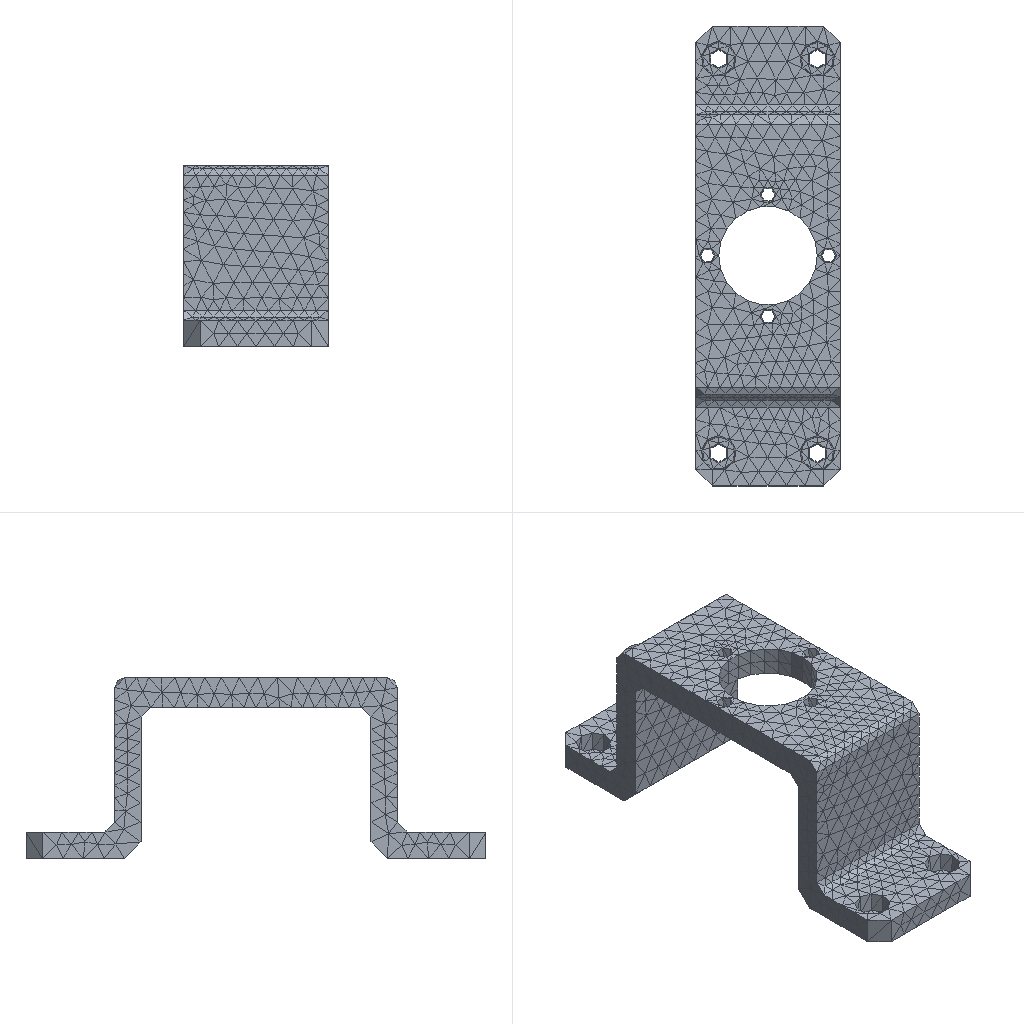Simulation study | nx simcenter
Set-up summary:
category,name,step,type,value,unit,region
solver,nx_nastran (Simcenter)
units,not stated in the deck,,not stated
analysis,deck,,static,static
analysis,solution,,SOL,101
load_step,SUBCASE 1,1,SUBCASE,SPC=1 LOAD=2
load_step,requested,,,1
mesh,nodes,,,9303
mesh,elements,,,4785
element_type,CTETRA,,solid,4785
load,nodal force total,,FX,0.0,model units
load,nodal force total,,FY,0.0,model units
load,nodal force total,,FZ,-1000000.057,model units
load,load commands in deck,,count,560
bc,support commands in deck,,count,508
analysis,NX solution 0,,Structural,Linear Statics - Single Constraint
check,setup vs results,,match,every grid point's frame and coordinates and every element id; grid points of CTETRA elements
Nastran input file, long lists of numbers shortened:
$*$$$$$$$$$$$$$$$$$$$$$$$$$$$$$$$$$$$$$$$$$$$$$$$$$$$$$$$$$$$$$$$$$
$*
$*                    NX v10.0.0.24 TRANSLATOR
$*                    FOR NX NASTRAN VERSION 10.0
$ (33 more lines like these left out)
ASSIGN OUTPUT2='143_sim1-solution_1.op2' UNIT=12
$*
$*$$$$$$$$$$$$$$$$$$$$$$$$$$$$$$$$$$$
$*
$* EXECUTIVE CONTROL
$*
$*$$$$$$$$$$$$$$$$$$$$$$$$$$$$$$$$$$$
$*
ID,NASTRAN,143_sim1-solution_1
SOL 101
CEND
$*
$*$$$$$$$$$$$$$$$$$$$$$$$$$$$$$$$$$$$
$*
$* CASE CONTROL
$*
$*$$$$$$$$$$$$$$$$$$$$$$$$$$$$$$$$$$$
$*
TITLE = Solution 1
ECHO = NONE
SPC = 1
OUTPUT
BCRESULTS(TRACTION,FORCE,PLOT) = ALL
DISPLACEMENT(PLOT) = ALL
ESE(PLOT) = ALL
FORCE(PLOT,CORNER) = ALL
OLOAD(PLOT) = ALL
SPCFORCES(PLOT) = ALL
STRAIN(PLOT,FIBER,CORNER) = ALL
STRESS(PLOT,CORNER) = ALL
$*  NX Step: Subcase - Static Loads 1
SUBCASE 1
LABEL = Subcase - Static Loads 1
LOAD = 2
$*
$*$$$$$$$$$$$$$$$$$$$$$$$$$$$$$$$$$$$
$*
$* BULK DATA
$*
$*$$$$$$$$$$$$$$$$$$$$$$$$$$$$$$$$$$$
$*
BEGIN BULK
$*
$* PARAM CARDS
$*
PARAM      K6ROT100.0000
PARAM     OIBULK     YES
PARAM    OMACHPR     YES
PARAM       POST      -2
PARAM    POSTEXT     YES
PARAM    UNITSYS   MN-MM
$*
$* GRID CARDS
$*
GRID*               9226               00.0000000000E+00-6.500000000E+01+
*       1.4541231446E-13               0
GRID*               9227               00.0000000000E+00-6.500000000E+01+
*       8.0000000000E+00               0
$ (18602 more lines like these left out)
$*
$* ELEMENT CARDS
$*
$*  NX Mesh Collector: Solid(1)
$*  NX Mesh: 3d_mesh(1)
CTETRA         1       1       1    6016    6017    8988     187    6419+
+            188     189    6417    6416
CTETRA         2       1       1    6012       2       3     190     191+
+            192     193     194     195
$ (9566 more lines like these left out)
$*
$* PROPERTY CARDS
$*
$*  NX Property: PSOLID1
PSOLID         1       1       0                           SMECH
$*
$* MATERIAL CARDS
$*
$*  NX Material: AISI_Steel_4340
MAT1           11.9300+8        0.2840007.8500-61.2300-5
$*
$* LOAD AND CONSTRAINT CARDS
$*
$*  NX Load and Constraint: Fixed(1)
SPC            1    7393  123456  0.0000
SPC            1    7394  123456  0.0000
SPC            1    7395  123456  0.0000
SPC            1    7396  123456  0.0000
$ (504 more lines like these left out)
$*  NX Load and Constraint: Force(1)
FORCE          2    6031       0724.5487  0.0000  0.0000-1.00000
FORCE          2    6032       0218.6753  0.0000  0.0000-1.00000
FORCE          2    6033       0 1296.20  0.0000  0.0000-1.00000
FORCE          2    6034       0534.2063  0.0000  0.0000-1.00000
$ (556 more lines like these left out)
ENDDATA 0de572b2
Results summary:
result,analysis,,,static
result,last_loadstep,,,1
result,primary field,,,displacements
result,reaction total,,FX,0.01702,model units
result,reaction total,,FY,-0.009284,model units
result,reaction total,,FZ,1000000.312,model units
result,NX solution 0,,loadcases,1,mm